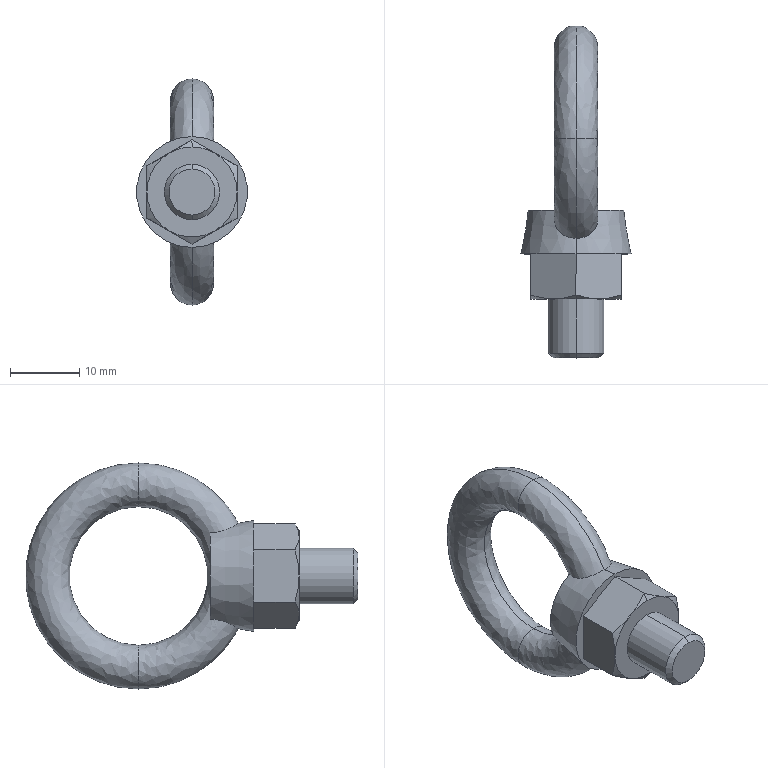Part | SolidWorks | features BaseBody 2 | 2 solids | 37 faces | box 16 x 47.95 x 32.6 mm | volume 4723 mm3 | cone 15 | plane 12 | spline 6 | cylinder 4 | commonest cylinder face diameters 6.647 x2 8 x2
STEP:
#1=CARTESIAN_POINT('',(0.,0.,-10.));
#2=VERTEX_POINT('',#1);
#3=CARTESIAN_POINT('',(0.,0.,10.));
#4=VERTEX_POINT('',#3);
#5=CARTESIAN_POINT('',(0.,0.,0.));
#6=DIRECTION('',(-1.,0.,0.));
#7=DIRECTION('',(0.,0.,1.));
#8=AXIS2_PLACEMENT_3D('',#5,#6,#7);
#9=CIRCLE('',#8,10.);
#10=EDGE_CURVE('',#2,#4,#9,.T.);
#11=ORIENTED_EDGE('',*,*,#10,.F.);
#12=CARTESIAN_POINT('',(0.,0.,-16.3));
#13=VERTEX_POINT('',#12);
#14=CARTESIAN_POINT('',(0.,0.,-13.15));
#15=DIRECTION('',(0.,-1.,0.));
#16=DIRECTION('',(0.,0.,-1.));
#17=AXIS2_PLACEMENT_3D('',#14,#15,#16);
#18=CIRCLE('',#17,3.15);
#19=EDGE_CURVE('',#2,#13,#18,.T.);
#20=ORIENTED_EDGE('',*,*,#19,.T.);
#21=CARTESIAN_POINT('',(0.,-14.417,-7.606));
#22=VERTEX_POINT('',#21);
#23=CARTESIAN_POINT('',(0.,0.,0.));
#24=DIRECTION('',(-1.,0.,0.));
#25=DIRECTION('',(0.,0.,1.));
#26=AXIS2_PLACEMENT_3D('',#23,#24,#25);
#27=CIRCLE('',#26,16.3);
#28=EDGE_CURVE('',#13,#22,#27,.T.);
#29=ORIENTED_EDGE('',*,*,#28,.T.);
#30=CARTESIAN_POINT('',(-2.961,-10.35,-6.22));
#31=VERTEX_POINT('',#30);
#32=CARTESIAN_POINT('',(0.,-14.417,-7.606));
#33=CARTESIAN_POINT('',(-0.2595,-14.417,-7.606));
#34=CARTESIAN_POINT('',(-0.5135,-14.39,-7.588));
#35=CARTESIAN_POINT('',(-1.011,-14.286,-7.52));
#36=CARTESIAN_POINT('',(-1.255,-14.207,-7.468));
#37=CARTESIAN_POINT('',(-1.594,-14.054,-7.373));
#38=CARTESIAN_POINT('',(-1.703,-13.996,-7.338));
#39=CARTESIAN_POINT('',(-1.913,-13.869,-7.263));
#40=CARTESIAN_POINT('',(-2.015,-13.799,-7.222));
#41=CARTESIAN_POINT('',(-2.302,-13.573,-7.096));
#42=CARTESIAN_POINT('',(-2.469,-13.402,-7.007));
#43=CARTESIAN_POINT('',(-2.757,-13.014,-6.825));
#44=CARTESIAN_POINT('',(-2.874,-12.801,-6.735));
#45=CARTESIAN_POINT('',(-3.047,-12.348,-6.57));
#46=CARTESIAN_POINT('',(-3.105,-12.104,-6.495));
#47=CARTESIAN_POINT('',(-3.158,-11.609,-6.372));
#48=CARTESIAN_POINT('',(-3.155,-11.354,-6.323));
#49=CARTESIAN_POINT('',(-3.096,-10.847,-6.252));
#50=CARTESIAN_POINT('',(-3.04,-10.597,-6.231));
#51=CARTESIAN_POINT('',(-2.961,-10.35,-6.22));
#52=B_SPLINE_CURVE_WITH_KNOTS('',3,(#32,#33,#34,#35,#36,#37,#38,#39,#40,#41,#42,#43,#44,#45,#46,#47,#48,#49,#50,#51),.UNSPECIFIED.,.F.,.F.,(4,2,2,2,2,2,2,2,2,4),(0.00614,0.006907,0.007674,0.008058,0.008441,0.009209,0.009976,0.01074,0.01151,0.01228),.UNSPECIFIED.);
#53=EDGE_CURVE('',#22,#31,#52,.T.);
#54=ORIENTED_EDGE('',*,*,#53,.T.);
#55=CARTESIAN_POINT('',(-2.961,-10.35,6.22));
#56=VERTEX_POINT('',#55);
#57=CARTESIAN_POINT('',(-2.961,-10.35,-6.22));
#58=CARTESIAN_POINT('',(-2.862,-10.35,-5.691));
#59=CARTESIAN_POINT('',(-2.732,-10.35,-5.171));
#60=CARTESIAN_POINT('',(-2.436,-10.35,-4.139));
#61=CARTESIAN_POINT('',(-2.271,-10.35,-3.628));
#62=CARTESIAN_POINT('',(-1.944,-10.35,-2.605));
#63=CARTESIAN_POINT('',(-1.78,-10.35,-2.093));
#64=CARTESIAN_POINT('',(-1.59,-10.35,-1.314));
#65=CARTESIAN_POINT('',(-1.537,-10.35,-1.052));
#66=CARTESIAN_POINT('',(-1.462,-10.35,-0.5207));
#67=CARTESIAN_POINT('',(-1.442,-10.35,-0.2495));
#68=CARTESIAN_POINT('',(-1.445,-10.35,0.5655));
#69=CARTESIAN_POINT('',(-1.534,-10.35,1.09));
#70=CARTESIAN_POINT('',(-1.789,-10.35,2.121));
#71=CARTESIAN_POINT('',(-1.952,-10.35,2.629));
#72=CARTESIAN_POINT('',(-2.277,-10.35,3.646));
#73=CARTESIAN_POINT('',(-2.441,-10.35,4.153));
#74=CARTESIAN_POINT('',(-2.733,-10.35,5.178));
#75=CARTESIAN_POINT('',(-2.863,-10.35,5.695));
#76=CARTESIAN_POINT('',(-2.961,-10.35,6.22));
#77=B_SPLINE_CURVE_WITH_KNOTS('',3,(#57,#58,#59,#60,#61,#62,#63,#64,#65,#66,#67,#68,#69,#70,#71,#72,#73,#74,#75,#76),.UNSPECIFIED.,.F.,.F.,(4,2,2,2,2,2,2,2,2,4),(0.,0.00161,0.003219,0.004829,0.005634,0.006439,0.008048,0.009658,0.01127,0.01288),.UNSPECIFIED.);
#78=EDGE_CURVE('',#31,#56,#77,.T.);
#79=ORIENTED_EDGE('',*,*,#78,.T.);
#80=CARTESIAN_POINT('',(0.,-14.417,7.606));
#81=VERTEX_POINT('',#80);
#82=CARTESIAN_POINT('',(-2.961,-10.35,6.22));
#83=CARTESIAN_POINT('',(-3.04,-10.596,6.231));
#84=CARTESIAN_POINT('',(-3.095,-10.846,6.252));
#85=CARTESIAN_POINT('',(-3.155,-11.35,6.322));
#86=CARTESIAN_POINT('',(-3.158,-11.607,6.371));
#87=CARTESIAN_POINT('',(-3.106,-12.1,6.493));
#88=CARTESIAN_POINT('',(-3.05,-12.34,6.567));
#89=CARTESIAN_POINT('',(-2.875,-12.798,6.734));
#90=CARTESIAN_POINT('',(-2.76,-13.009,6.823));
#91=CARTESIAN_POINT('',(-2.546,-13.299,6.959));
#92=CARTESIAN_POINT('',(-2.466,-13.392,7.005));
#93=CARTESIAN_POINT('',(-2.298,-13.566,7.094));
#94=CARTESIAN_POINT('',(-2.208,-13.646,7.137));
#95=CARTESIAN_POINT('',(-1.923,-13.872,7.263));
#96=CARTESIAN_POINT('',(-1.709,-14.001,7.34));
#97=CARTESIAN_POINT('',(-1.257,-14.206,7.468));
#98=CARTESIAN_POINT('',(-1.017,-14.285,7.519));
#99=CARTESIAN_POINT('',(-0.5148,-14.39,7.588));
#100=CARTESIAN_POINT('',(-0.2595,-14.417,7.606));
#101=CARTESIAN_POINT('',(0.,-14.417,7.606));
#102=B_SPLINE_CURVE_WITH_KNOTS('',3,(#82,#83,#84,#85,#86,#87,#88,#89,#90,#91,#92,#93,#94,#95,#96,#97,#98,#99,#100,#101),.UNSPECIFIED.,.F.,.F.,(4,2,2,2,2,2,2,2,2,4),(-0.00614,-0.005372,-0.004605,-0.003837,-0.00307,-0.002686,-0.002302,-0.001535,-0.0007674,0.),.UNSPECIFIED.);
#103=EDGE_CURVE('',#56,#81,#102,.T.);
#104=ORIENTED_EDGE('',*,*,#103,.T.);
#105=CARTESIAN_POINT('',(0.,0.,16.3));
#106=VERTEX_POINT('',#105);
#107=CARTESIAN_POINT('',(0.,0.,0.));
#108=DIRECTION('',(-1.,0.,0.));
#109=DIRECTION('',(0.,0.,1.));
#110=AXIS2_PLACEMENT_3D('',#107,#108,#109);
#111=CIRCLE('',#110,16.3);
#112=EDGE_CURVE('',#81,#106,#111,.T.);
#113=ORIENTED_EDGE('',*,*,#112,.T.);
#114=CARTESIAN_POINT('',(0.,0.,13.15));
#115=DIRECTION('',(0.,1.,0.));
#116=DIRECTION('',(0.,0.,1.));
#117=AXIS2_PLACEMENT_3D('',#114,#115,#116);
#118=CIRCLE('',#117,3.15);
#119=EDGE_CURVE('',#4,#106,#118,.T.);
#120=ORIENTED_EDGE('',*,*,#119,.F.);
#121=EDGE_LOOP('',(#11,#20,#29,#54,#79,#104,#113,#120));
#122=FACE_OUTER_BOUND('',#121,.T.);
#123=CARTESIAN_POINT('',(0.,0.,-10.));
#124=CARTESIAN_POINT('',(0.,-20.,-10.));
#125=CARTESIAN_POINT('',(0.,-20.,10.));
#126=CARTESIAN_POINT('',(0.,0.,10.));
#127=CARTESIAN_POINT('',(-6.3,0.,-10.));
#128=CARTESIAN_POINT('',(-6.3,-20.,-10.));
#129=CARTESIAN_POINT('',(-6.3,-20.,10.));
#130=CARTESIAN_POINT('',(-6.3,0.,10.));
#131=CARTESIAN_POINT('',(-6.3,0.,-16.3));
#132=CARTESIAN_POINT('',(-6.3,-32.6,-16.3));
#133=CARTESIAN_POINT('',(-6.3,-32.6,16.3));
#134=CARTESIAN_POINT('',(-6.3,0.,16.3));
#135=CARTESIAN_POINT('',(0.,0.,-16.3));
#136=CARTESIAN_POINT('',(0.,-32.6,-16.3));
#137=CARTESIAN_POINT('',(0.,-32.6,16.3));
#138=CARTESIAN_POINT('',(0.,0.,16.3));
#139=(BOUNDED_SURFACE()B_SPLINE_SURFACE(3,3,((#123,#124,#125,#126),(#127,#128,#129,#130),(#131,#132,#133,#134),(#135,#136,#137,#138)),.UNSPECIFIED.,.F.,.F.,.F.)B_SPLINE_SURFACE_WITH_KNOTS((4,4),(4,4),(0.,1.),(0.,1.),.UNSPECIFIED.)GEOMETRIC_REPRESENTATION_ITEM()RATIONAL_B_SPLINE_SURFACE(((1.,0.3333,0.3333,1.),(0.3333,0.1111,0.1111,0.3333),(0.3333,0.1111,0.1111,0.3333),(1.,0.3333,0.3333,1.)))REPRESENTATION_ITEM('')SURFACE());
#140=ADVANCED_FACE('',(#122),#139,.T.);
#141=CARTESIAN_POINT('',(0.,-19.65,-4.));
#142=VERTEX_POINT('',#141);
#143=CARTESIAN_POINT('',(0.,-19.65,4.));
#144=VERTEX_POINT('',#143);
#145=CARTESIAN_POINT('',(0.,-19.65,0.));
#146=DIRECTION('',(0.,-1.,0.));
#147=DIRECTION('',(0.,0.,1.));
#148=AXIS2_PLACEMENT_3D('',#145,#146,#147);
#149=CIRCLE('',#148,4.);
#150=EDGE_CURVE('',#142,#144,#149,.T.);
#151=ORIENTED_EDGE('',*,*,#150,.F.);
#152=CARTESIAN_POINT('',(0.,-16.65,-4.));
#153=VERTEX_POINT('',#152);
#154=CARTESIAN_POINT('',(0.,-18.15,-7.708));
#155=DIRECTION('',(-1.,0.,0.));
#156=DIRECTION('',(0.,0.,-1.));
#157=AXIS2_PLACEMENT_3D('',#154,#155,#156);
#158=CIRCLE('',#157,4.);
#159=EDGE_CURVE('',#142,#153,#158,.T.);
#160=ORIENTED_EDGE('',*,*,#159,.T.);
#161=CARTESIAN_POINT('',(0.,-16.65,4.));
#162=VERTEX_POINT('',#161);
#163=CARTESIAN_POINT('',(0.,-16.65,0.));
#164=DIRECTION('',(0.,1.,0.));
#165=DIRECTION('',(0.,0.,1.));
#166=AXIS2_PLACEMENT_3D('',#163,#164,#165);
#167=CIRCLE('',#166,4.);
#168=EDGE_CURVE('',#162,#153,#167,.T.);
#169=ORIENTED_EDGE('',*,*,#168,.F.);
#170=CARTESIAN_POINT('',(0.,-18.15,7.708));
#171=DIRECTION('',(1.,0.,0.));
#172=DIRECTION('',(0.,0.,1.));
#173=AXIS2_PLACEMENT_3D('',#170,#171,#172);
#174=CIRCLE('',#173,4.);
#175=EDGE_CURVE('',#144,#162,#174,.T.);
#176=ORIENTED_EDGE('',*,*,#175,.F.);
#177=EDGE_LOOP('',(#151,#160,#169,#176));
#178=FACE_OUTER_BOUND('',#177,.T.);
#179=CARTESIAN_POINT('',(0.,-19.65,4.));
#180=CARTESIAN_POINT('',(8.,-19.65,4.));
#181=CARTESIAN_POINT('',(8.,-19.65,-4.));
#182=CARTESIAN_POINT('',(0.,-19.65,-4.));
#183=CARTESIAN_POINT('',(0.,-18.676,3.606));
#184=CARTESIAN_POINT('',(7.212,-18.676,3.606));
#185=CARTESIAN_POINT('',(7.212,-18.676,-3.606));
#186=CARTESIAN_POINT('',(0.,-18.676,-3.606));
#187=CARTESIAN_POINT('',(0.,-17.624,3.606));
#188=CARTESIAN_POINT('',(7.212,-17.624,3.606));
#189=CARTESIAN_POINT('',(7.212,-17.624,-3.606));
#190=CARTESIAN_POINT('',(0.,-17.624,-3.606));
#191=CARTESIAN_POINT('',(0.,-16.65,4.));
#192=CARTESIAN_POINT('',(8.,-16.65,4.));
#193=CARTESIAN_POINT('',(8.,-16.65,-4.));
#194=CARTESIAN_POINT('',(0.,-16.65,-4.));
#195=(BOUNDED_SURFACE()B_SPLINE_SURFACE(3,3,((#179,#180,#181,#182),(#183,#184,#185,#186),(#187,#188,#189,#190),(#191,#192,#193,#194)),.UNSPECIFIED.,.F.,.F.,.F.)B_SPLINE_SURFACE_WITH_KNOTS((4,4),(4,4),(0.,1.),(0.,1.),.UNSPECIFIED.)GEOMETRIC_REPRESENTATION_ITEM()RATIONAL_B_SPLINE_SURFACE(((1.,0.3333,0.3333,1.),(0.9513,0.3171,0.3171,0.9513),(0.9513,0.3171,0.3171,0.9513),(1.,0.3333,0.3333,1.)))REPRESENTATION_ITEM('')SURFACE());
#196=ADVANCED_FACE('',(#178),#195,.F.);
#197=ORIENTED_EDGE('',*,*,#28,.F.);
#198=CARTESIAN_POINT('',(0.,0.,-13.15));
#199=DIRECTION('',(0.,-1.,0.));
#200=DIRECTION('',(0.,0.,-1.));
#201=AXIS2_PLACEMENT_3D('',#198,#199,#200);
#202=CIRCLE('',#201,3.15);
#203=EDGE_CURVE('',#13,#2,#202,.T.);
#204=ORIENTED_EDGE('',*,*,#203,.T.);
#205=ORIENTED_EDGE('',*,*,#10,.T.);
#206=CARTESIAN_POINT('',(0.,0.,13.15));
#207=DIRECTION('',(0.,1.,0.));
#208=DIRECTION('',(0.,0.,1.));
#209=AXIS2_PLACEMENT_3D('',#206,#207,#208);
#210=CIRCLE('',#209,3.15);
#211=EDGE_CURVE('',#106,#4,#210,.T.);
#212=ORIENTED_EDGE('',*,*,#211,.F.);
#213=ORIENTED_EDGE('',*,*,#112,.F.);
#214=CARTESIAN_POINT('',(2.961,-10.35,6.22));
#215=VERTEX_POINT('',#214);
#216=CARTESIAN_POINT('',(0.,-14.417,7.606));
#217=CARTESIAN_POINT('',(0.2595,-14.417,7.606));
#218=CARTESIAN_POINT('',(0.5135,-14.39,7.588));
#219=CARTESIAN_POINT('',(1.011,-14.286,7.52));
#220=CARTESIAN_POINT('',(1.255,-14.207,7.468));
#221=CARTESIAN_POINT('',(1.594,-14.054,7.373));
#222=CARTESIAN_POINT('',(1.703,-13.996,7.338));
#223=CARTESIAN_POINT('',(1.913,-13.869,7.263));
#224=CARTESIAN_POINT('',(2.015,-13.799,7.222));
#225=CARTESIAN_POINT('',(2.302,-13.573,7.096));
#226=CARTESIAN_POINT('',(2.469,-13.402,7.007));
#227=CARTESIAN_POINT('',(2.757,-13.014,6.825));
#228=CARTESIAN_POINT('',(2.874,-12.801,6.735));
#229=CARTESIAN_POINT('',(3.047,-12.348,6.57));
#230=CARTESIAN_POINT('',(3.105,-12.104,6.495));
#231=CARTESIAN_POINT('',(3.158,-11.609,6.372));
#232=CARTESIAN_POINT('',(3.155,-11.354,6.323));
#233=CARTESIAN_POINT('',(3.096,-10.847,6.252));
#234=CARTESIAN_POINT('',(3.04,-10.597,6.231));
#235=CARTESIAN_POINT('',(2.961,-10.35,6.22));
#236=B_SPLINE_CURVE_WITH_KNOTS('',3,(#216,#217,#218,#219,#220,#221,#222,#223,#224,#225,#226,#227,#228,#229,#230,#231,#232,#233,#234,#235),.UNSPECIFIED.,.F.,.F.,(4,2,2,2,2,2,2,2,2,4),(0.,0.0007672,0.001534,0.001918,0.002302,0.003069,0.003836,0.004603,0.005371,0.006138),.UNSPECIFIED.);
#237=EDGE_CURVE('',#81,#215,#236,.T.);
#238=ORIENTED_EDGE('',*,*,#237,.T.);
#239=CARTESIAN_POINT('',(2.961,-10.35,-6.22));
#240=VERTEX_POINT('',#239);
#241=CARTESIAN_POINT('',(2.961,-10.35,6.22));
#242=CARTESIAN_POINT('',(2.862,-10.35,5.691));
#243=CARTESIAN_POINT('',(2.732,-10.35,5.171));
#244=CARTESIAN_POINT('',(2.436,-10.35,4.139));
#245=CARTESIAN_POINT('',(2.271,-10.35,3.628));
#246=CARTESIAN_POINT('',(1.944,-10.35,2.605));
#247=CARTESIAN_POINT('',(1.78,-10.35,2.093));
#248=CARTESIAN_POINT('',(1.59,-10.35,1.314));
#249=CARTESIAN_POINT('',(1.537,-10.35,1.052));
#250=CARTESIAN_POINT('',(1.462,-10.35,0.5207));
#251=CARTESIAN_POINT('',(1.442,-10.35,0.2495));
#252=CARTESIAN_POINT('',(1.445,-10.35,-0.5655));
#253=CARTESIAN_POINT('',(1.534,-10.35,-1.09));
#254=CARTESIAN_POINT('',(1.789,-10.35,-2.121));
#255=CARTESIAN_POINT('',(1.952,-10.35,-2.629));
#256=CARTESIAN_POINT('',(2.277,-10.35,-3.646));
#257=CARTESIAN_POINT('',(2.441,-10.35,-4.153));
#258=CARTESIAN_POINT('',(2.733,-10.35,-5.178));
#259=CARTESIAN_POINT('',(2.863,-10.35,-5.695));
#260=CARTESIAN_POINT('',(2.961,-10.35,-6.22));
#261=B_SPLINE_CURVE_WITH_KNOTS('',3,(#241,#242,#243,#244,#245,#246,#247,#248,#249,#250,#251,#252,#253,#254,#255,#256,#257,#258,#259,#260),.UNSPECIFIED.,.F.,.F.,(4,2,2,2,2,2,2,2,2,4),(0.,0.00161,0.003219,0.004829,0.005634,0.006439,0.008048,0.009658,0.01127,0.01288),.UNSPECIFIED.);
#262=EDGE_CURVE('',#215,#240,#261,.T.);
#263=ORIENTED_EDGE('',*,*,#262,.T.);
#264=CARTESIAN_POINT('',(2.961,-10.35,-6.22));
#265=CARTESIAN_POINT('',(3.04,-10.596,-6.231));
#266=CARTESIAN_POINT('',(3.095,-10.846,-6.252));
#267=CARTESIAN_POINT('',(3.155,-11.35,-6.322));
#268=CARTESIAN_POINT('',(3.158,-11.607,-6.371));
#269=CARTESIAN_POINT('',(3.106,-12.1,-6.493));
#270=CARTESIAN_POINT('',(3.05,-12.34,-6.567));
#271=CARTESIAN_POINT('',(2.875,-12.798,-6.734));
#272=CARTESIAN_POINT('',(2.76,-13.009,-6.823));
#273=CARTESIAN_POINT('',(2.546,-13.299,-6.959));
#274=CARTESIAN_POINT('',(2.466,-13.392,-7.005));
#275=CARTESIAN_POINT('',(2.298,-13.566,-7.094));
#276=CARTESIAN_POINT('',(2.208,-13.646,-7.137));
#277=CARTESIAN_POINT('',(1.923,-13.872,-7.263));
#278=CARTESIAN_POINT('',(1.709,-14.001,-7.34));
#279=CARTESIAN_POINT('',(1.257,-14.206,-7.468));
#280=CARTESIAN_POINT('',(1.017,-14.285,-7.519));
#281=CARTESIAN_POINT('',(0.5148,-14.39,-7.588));
#282=CARTESIAN_POINT('',(0.2595,-14.417,-7.606));
#283=CARTESIAN_POINT('',(0.,-14.417,-7.606));
#284=B_SPLINE_CURVE_WITH_KNOTS('',3,(#264,#265,#266,#267,#268,#269,#270,#271,#272,#273,#274,#275,#276,#277,#278,#279,#280,#281,#282,#283),.UNSPECIFIED.,.F.,.F.,(4,2,2,2,2,2,2,2,2,4),(0.,0.0007675,0.001535,0.002302,0.00307,0.003454,0.003837,0.004605,0.005372,0.00614),.UNSPECIFIED.);
#285=EDGE_CURVE('',#240,#22,#284,.T.);
#286=ORIENTED_EDGE('',*,*,#285,.T.);
#287=EDGE_LOOP('',(#197,#204,#205,#212,#213,#238,#263,#286));
#288=FACE_OUTER_BOUND('',#287,.T.);
#289=CARTESIAN_POINT('',(0.,0.,-16.3));
#290=CARTESIAN_POINT('',(0.,-32.6,-16.3));
#291=CARTESIAN_POINT('',(0.,-32.6,16.3));
#292=CARTESIAN_POINT('',(0.,0.,16.3));
#293=CARTESIAN_POINT('',(6.3,0.,-16.3));
#294=CARTESIAN_POINT('',(6.3,-32.6,-16.3));
#295=CARTESIAN_POINT('',(6.3,-32.6,16.3));
#296=CARTESIAN_POINT('',(6.3,0.,16.3));
#297=CARTESIAN_POINT('',(6.3,0.,-10.));
#298=CARTESIAN_POINT('',(6.3,-20.,-10.));
#299=CARTESIAN_POINT('',(6.3,-20.,10.));
#300=CARTESIAN_POINT('',(6.3,0.,10.));
#301=CARTESIAN_POINT('',(0.,0.,-10.));
#302=CARTESIAN_POINT('',(0.,-20.,-10.));
#303=CARTESIAN_POINT('',(0.,-20.,10.));
#304=CARTESIAN_POINT('',(0.,0.,10.));
#305=(BOUNDED_SURFACE()B_SPLINE_SURFACE(3,3,((#289,#290,#291,#292),(#293,#294,#295,#296),(#297,#298,#299,#300),(#301,#302,#303,#304)),.UNSPECIFIED.,.F.,.F.,.F.)B_SPLINE_SURFACE_WITH_KNOTS((4,4),(4,4),(0.,1.),(0.,1.),.UNSPECIFIED.)GEOMETRIC_REPRESENTATION_ITEM()RATIONAL_B_SPLINE_SURFACE(((1.,0.3333,0.3333,1.),(0.3333,0.1111,0.1111,0.3333),(0.3333,0.1111,0.1111,0.3333),(1.,0.3333,0.3333,1.)))REPRESENTATION_ITEM('')SURFACE());
#306=ADVANCED_FACE('',(#288),#305,.T.);
#307=ORIENTED_EDGE('',*,*,#203,.F.);
#308=CARTESIAN_POINT('',(0.,0.,0.));
#309=DIRECTION('',(-1.,0.,0.));
#310=DIRECTION('',(0.,0.,1.));
#311=AXIS2_PLACEMENT_3D('',#308,#309,#310);
#312=CIRCLE('',#311,16.3);
#313=EDGE_CURVE('',#106,#13,#312,.T.);
#314=ORIENTED_EDGE('',*,*,#313,.F.);
#315=ORIENTED_EDGE('',*,*,#211,.T.);
#316=CARTESIAN_POINT('',(0.,0.,0.));
#317=DIRECTION('',(-1.,0.,0.));
#318=DIRECTION('',(0.,0.,1.));
#319=AXIS2_PLACEMENT_3D('',#316,#317,#318);
#320=CIRCLE('',#319,10.);
#321=EDGE_CURVE('',#4,#2,#320,.T.);
#322=ORIENTED_EDGE('',*,*,#321,.T.);
#323=EDGE_LOOP('',(#307,#314,#315,#322));
#324=FACE_OUTER_BOUND('',#323,.T.);
#325=CARTESIAN_POINT('',(0.,0.,16.3));
#326=CARTESIAN_POINT('',(0.,32.6,16.3));
#327=CARTESIAN_POINT('',(0.,32.6,-16.3));
#328=CARTESIAN_POINT('',(0.,0.,-16.3));
#329=CARTESIAN_POINT('',(6.3,0.,16.3));
#330=CARTESIAN_POINT('',(6.3,32.6,16.3));
#331=CARTESIAN_POINT('',(6.3,32.6,-16.3));
#332=CARTESIAN_POINT('',(6.3,0.,-16.3));
#333=CARTESIAN_POINT('',(6.3,0.,10.));
#334=CARTESIAN_POINT('',(6.3,20.,10.));
#335=CARTESIAN_POINT('',(6.3,20.,-10.));
#336=CARTESIAN_POINT('',(6.3,0.,-10.));
#337=CARTESIAN_POINT('',(0.,0.,10.));
#338=CARTESIAN_POINT('',(0.,20.,10.));
#339=CARTESIAN_POINT('',(0.,20.,-10.));
#340=CARTESIAN_POINT('',(0.,0.,-10.));
#341=(BOUNDED_SURFACE()B_SPLINE_SURFACE(3,3,((#325,#326,#327,#328),(#329,#330,#331,#332),(#333,#334,#335,#336),(#337,#338,#339,#340)),.UNSPECIFIED.,.F.,.F.,.F.)B_SPLINE_SURFACE_WITH_KNOTS((4,4),(4,4),(0.,1.),(0.,1.),.UNSPECIFIED.)GEOMETRIC_REPRESENTATION_ITEM()RATIONAL_B_SPLINE_SURFACE(((1.,0.3333,0.3333,1.),(0.3333,0.1111,0.1111,0.3333),(0.3333,0.1111,0.1111,0.3333),(1.,0.3333,0.3333,1.)))REPRESENTATION_ITEM('')SURFACE());
#342=ADVANCED_FACE('',(#324),#341,.T.);
#343=ORIENTED_EDGE('',*,*,#237,.F.);
#344=CARTESIAN_POINT('',(0.,-16.65,8.));
#345=VERTEX_POINT('',#344);
#346=CARTESIAN_POINT('',(0.,-16.65,8.));
#347=DIRECTION('',(0.,-0.9848,0.1736));
#348=VECTOR('',#347,1000.);
#349=LINE('',#346,#348);
#350=EDGE_CURVE('',#81,#345,#349,.T.);
#351=ORIENTED_EDGE('',*,*,#350,.T.);
#352=CARTESIAN_POINT('',(0.,-16.65,-8.));
#353=VERTEX_POINT('',#352);
#354=CARTESIAN_POINT('',(0.,-16.65,0.));
#355=DIRECTION('',(0.,1.,0.));
#356=DIRECTION('',(0.,0.,-1.));
#357=AXIS2_PLACEMENT_3D('',#354,#355,#356);
#358=CIRCLE('',#357,8.);
#359=EDGE_CURVE('',#345,#353,#358,.T.);
#360=ORIENTED_EDGE('',*,*,#359,.T.);
#361=CARTESIAN_POINT('',(0.,-16.65,-8.));
#362=DIRECTION('',(0.,-0.9848,-0.1736));
#363=VECTOR('',#362,1000.);
#364=LINE('',#361,#363);
#365=EDGE_CURVE('',#22,#353,#364,.T.);
#366=ORIENTED_EDGE('',*,*,#365,.F.);
#367=ORIENTED_EDGE('',*,*,#285,.F.);
#368=CARTESIAN_POINT('',(0.,-10.35,0.));
#369=DIRECTION('',(0.,-1.,0.));
#370=DIRECTION('',(0.,0.,-1.));
#371=AXIS2_PLACEMENT_3D('',#368,#369,#370);
#372=CIRCLE('',#371,6.889);
#373=EDGE_CURVE('',#240,#215,#372,.T.);
#374=ORIENTED_EDGE('',*,*,#373,.T.);
#375=EDGE_LOOP('',(#343,#351,#360,#366,#367,#374));
#376=FACE_OUTER_BOUND('',#375,.T.);
#377=CARTESIAN_POINT('',(0.,-16.65,0.));
#378=DIRECTION('',(0.,-1.,0.));
#379=DIRECTION('',(0.,0.,-1.));
#380=AXIS2_PLACEMENT_3D('',#377,#378,#379);
#381=CONICAL_SURFACE('',#380,8.,0.1745);
#382=ADVANCED_FACE('',(#376),#381,.T.);
#383=ORIENTED_EDGE('',*,*,#150,.T.);
#384=CARTESIAN_POINT('',(0.,-30.974,4.));
#385=VERTEX_POINT('',#384);
#386=CARTESIAN_POINT('',(0.,-25.312,4.));
#387=DIRECTION('',(0.,-1.,0.));
#388=VECTOR('',#387,1000.);
#389=LINE('',#386,#388);
#390=EDGE_CURVE('',#144,#385,#389,.T.);
#391=ORIENTED_EDGE('',*,*,#390,.T.);
#392=CARTESIAN_POINT('',(0.,-30.974,-4.));
#393=VERTEX_POINT('',#392);
#394=CARTESIAN_POINT('',(0.,-30.974,0.));
#395=DIRECTION('',(0.,1.,0.));
#396=DIRECTION('',(0.,0.,-1.));
#397=AXIS2_PLACEMENT_3D('',#394,#395,#396);
#398=CIRCLE('',#397,4.);
#399=EDGE_CURVE('',#385,#393,#398,.T.);
#400=ORIENTED_EDGE('',*,*,#399,.T.);
#401=CARTESIAN_POINT('',(0.,-25.312,-4.));
#402=DIRECTION('',(0.,-1.,0.));
#403=VECTOR('',#402,1000.);
#404=LINE('',#401,#403);
#405=EDGE_CURVE('',#142,#393,#404,.T.);
#406=ORIENTED_EDGE('',*,*,#405,.F.);
#407=EDGE_LOOP('',(#383,#391,#400,#406));
#408=FACE_OUTER_BOUND('',#407,.T.);
#409=CARTESIAN_POINT('',(0.,-25.312,0.));
#410=DIRECTION('',(0.,-1.,0.));
#411=DIRECTION('',(0.,0.,-1.));
#412=AXIS2_PLACEMENT_3D('',#409,#410,#411);
#413=CYLINDRICAL_SURFACE('',#412,4.);
#414=ADVANCED_FACE('',(#408),#413,.T.);
#415=CARTESIAN_POINT('',(0.,-31.65,3.324));
#416=VERTEX_POINT('',#415);
#417=CARTESIAN_POINT('',(0.,-31.65,-3.324));
#418=VERTEX_POINT('',#417);
#419=CARTESIAN_POINT('',(0.,-31.65,0.));
#420=DIRECTION('',(0.,1.,0.));
#421=DIRECTION('',(0.,0.,1.));
#422=AXIS2_PLACEMENT_3D('',#419,#420,#421);
#423=CIRCLE('',#422,3.324);
#424=EDGE_CURVE('',#416,#418,#423,.T.);
#425=ORIENTED_EDGE('',*,*,#424,.T.);
#426=CARTESIAN_POINT('',(0.,-30.974,-4.));
#427=DIRECTION('',(0.,0.7071,-0.7071));
#428=VECTOR('',#427,1000.);
#429=LINE('',#426,#428);
#430=EDGE_CURVE('',#418,#393,#429,.T.);
#431=ORIENTED_EDGE('',*,*,#430,.T.);
#432=ORIENTED_EDGE('',*,*,#399,.F.);
#433=CARTESIAN_POINT('',(0.,-30.974,4.));
#434=DIRECTION('',(0.,0.7071,0.7071));
#435=VECTOR('',#434,1000.);
#436=LINE('',#433,#435);
#437=EDGE_CURVE('',#416,#385,#436,.T.);
#438=ORIENTED_EDGE('',*,*,#437,.F.);
#439=EDGE_LOOP('',(#425,#431,#432,#438));
#440=FACE_OUTER_BOUND('',#439,.T.);
#441=CARTESIAN_POINT('',(0.,-30.974,0.));
#442=DIRECTION('',(0.,1.,0.));
#443=DIRECTION('',(0.,0.,1.));
#444=AXIS2_PLACEMENT_3D('',#441,#442,#443);
#445=CONICAL_SURFACE('',#444,4.,0.7854);
#446=ADVANCED_FACE('',(#440),#445,.T.);
#447=ORIENTED_EDGE('',*,*,#19,.F.);
#448=ORIENTED_EDGE('',*,*,#321,.F.);
#449=ORIENTED_EDGE('',*,*,#119,.T.);
#450=ORIENTED_EDGE('',*,*,#313,.T.);
#451=EDGE_LOOP('',(#447,#448,#449,#450));
#452=FACE_OUTER_BOUND('',#451,.T.);
#453=CARTESIAN_POINT('',(0.,0.,10.));
#454=CARTESIAN_POINT('',(0.,20.,10.));
#455=CARTESIAN_POINT('',(0.,20.,-10.));
#456=CARTESIAN_POINT('',(0.,0.,-10.));
#457=CARTESIAN_POINT('',(-6.3,0.,10.));
#458=CARTESIAN_POINT('',(-6.3,20.,10.));
#459=CARTESIAN_POINT('',(-6.3,20.,-10.));
#460=CARTESIAN_POINT('',(-6.3,0.,-10.));
#461=CARTESIAN_POINT('',(-6.3,0.,16.3));
#462=CARTESIAN_POINT('',(-6.3,32.6,16.3));
#463=CARTESIAN_POINT('',(-6.3,32.6,-16.3));
#464=CARTESIAN_POINT('',(-6.3,0.,-16.3));
#465=CARTESIAN_POINT('',(0.,0.,16.3));
#466=CARTESIAN_POINT('',(0.,32.6,16.3));
#467=CARTESIAN_POINT('',(0.,32.6,-16.3));
#468=CARTESIAN_POINT('',(0.,0.,-16.3));
#469=(BOUNDED_SURFACE()B_SPLINE_SURFACE(3,3,((#453,#454,#455,#456),(#457,#458,#459,#460),(#461,#462,#463,#464),(#465,#466,#467,#468)),.UNSPECIFIED.,.F.,.F.,.F.)B_SPLINE_SURFACE_WITH_KNOTS((4,4),(4,4),(0.,1.),(0.,1.),.UNSPECIFIED.)GEOMETRIC_REPRESENTATION_ITEM()RATIONAL_B_SPLINE_SURFACE(((1.,0.3333,0.3333,1.),(0.3333,0.1111,0.1111,0.3333),(0.3333,0.1111,0.1111,0.3333),(1.,0.3333,0.3333,1.)))REPRESENTATION_ITEM('')SURFACE());
#470=ADVANCED_FACE('',(#452),#469,.T.);
#471=ORIENTED_EDGE('',*,*,#350,.F.);
#472=ORIENTED_EDGE('',*,*,#103,.F.);
#473=CARTESIAN_POINT('',(0.,-10.35,0.));
#474=DIRECTION('',(0.,-1.,0.));
#475=DIRECTION('',(0.,0.,-1.));
#476=AXIS2_PLACEMENT_3D('',#473,#474,#475);
#477=CIRCLE('',#476,6.889);
#478=EDGE_CURVE('',#56,#31,#477,.T.);
#479=ORIENTED_EDGE('',*,*,#478,.T.);
#480=ORIENTED_EDGE('',*,*,#53,.F.);
#481=ORIENTED_EDGE('',*,*,#365,.T.);
#482=CARTESIAN_POINT('',(0.,-16.65,0.));
#483=DIRECTION('',(0.,1.,0.));
#484=DIRECTION('',(0.,0.,-1.));
#485=AXIS2_PLACEMENT_3D('',#482,#483,#484);
#486=CIRCLE('',#485,8.);
#487=EDGE_CURVE('',#353,#345,#486,.T.);
#488=ORIENTED_EDGE('',*,*,#487,.T.);
#489=EDGE_LOOP('',(#471,#472,#479,#480,#481,#488));
#490=FACE_OUTER_BOUND('',#489,.T.);
#491=CARTESIAN_POINT('',(0.,-16.65,0.));
#492=DIRECTION('',(0.,-1.,0.));
#493=DIRECTION('',(0.,0.,-1.));
#494=AXIS2_PLACEMENT_3D('',#491,#492,#493);
#495=CONICAL_SURFACE('',#494,8.,0.1745);
#496=ADVANCED_FACE('',(#490),#495,.T.);
#497=ORIENTED_EDGE('',*,*,#262,.F.);
#498=ORIENTED_EDGE('',*,*,#373,.F.);
#499=EDGE_LOOP('',(#497,#498));
#500=FACE_OUTER_BOUND('',#499,.T.);
#501=CARTESIAN_POINT('',(0.,-10.35,-3.445));
#502=DIRECTION('',(0.,1.,0.));
#503=DIRECTION('',(0.,0.,1.));
#504=AXIS2_PLACEMENT_3D('',#501,#502,#503);
#505=PLANE('',#504);
#506=ADVANCED_FACE('',(#500),#505,.T.);
#507=ORIENTED_EDGE('',*,*,#78,.F.);
#508=ORIENTED_EDGE('',*,*,#478,.F.);
#509=EDGE_LOOP('',(#507,#508));
#510=FACE_OUTER_BOUND('',#509,.T.);
#511=CARTESIAN_POINT('',(0.,-10.35,-3.445));
#512=DIRECTION('',(0.,1.,0.));
#513=DIRECTION('',(0.,0.,1.));
#514=AXIS2_PLACEMENT_3D('',#511,#512,#513);
#515=PLANE('',#514);
#516=ADVANCED_FACE('',(#510),#515,.T.);
#517=ORIENTED_EDGE('',*,*,#168,.T.);
#518=CARTESIAN_POINT('',(0.,-16.65,0.));
#519=DIRECTION('',(0.,1.,0.));
#520=DIRECTION('',(0.,0.,1.));
#521=AXIS2_PLACEMENT_3D('',#518,#519,#520);
#522=CIRCLE('',#521,4.);
#523=EDGE_CURVE('',#153,#162,#522,.T.);
#524=ORIENTED_EDGE('',*,*,#523,.T.);
#525=EDGE_LOOP('',(#517,#524));
#526=FACE_BOUND('',#525,.T.);
#527=ORIENTED_EDGE('',*,*,#487,.F.);
#528=ORIENTED_EDGE('',*,*,#359,.F.);
#529=EDGE_LOOP('',(#527,#528));
#530=FACE_OUTER_BOUND('',#529,.T.);
#531=CARTESIAN_POINT('',(0.,-16.65,-6.));
#532=DIRECTION('',(0.,-1.,0.));
#533=DIRECTION('',(0.,0.,-1.));
#534=AXIS2_PLACEMENT_3D('',#531,#532,#533);
#535=PLANE('',#534);
#536=ADVANCED_FACE('',(#526,#530),#535,.T.);
#537=ORIENTED_EDGE('',*,*,#159,.F.);
#538=CARTESIAN_POINT('',(0.,-19.65,0.));
#539=DIRECTION('',(0.,-1.,0.));
#540=DIRECTION('',(0.,0.,1.));
#541=AXIS2_PLACEMENT_3D('',#538,#539,#540);
#542=CIRCLE('',#541,4.);
#543=EDGE_CURVE('',#144,#142,#542,.T.);
#544=ORIENTED_EDGE('',*,*,#543,.F.);
#545=ORIENTED_EDGE('',*,*,#175,.T.);
#546=ORIENTED_EDGE('',*,*,#523,.F.);
#547=EDGE_LOOP('',(#537,#544,#545,#546));
#548=FACE_OUTER_BOUND('',#547,.T.);
#549=CARTESIAN_POINT('',(0.,-19.65,-4.));
#550=CARTESIAN_POINT('',(-8.,-19.65,-4.));
#551=CARTESIAN_POINT('',(-8.,-19.65,4.));
#552=CARTESIAN_POINT('',(0.,-19.65,4.));
#553=CARTESIAN_POINT('',(0.,-18.676,-3.606));
#554=CARTESIAN_POINT('',(-7.212,-18.676,-3.606));
#555=CARTESIAN_POINT('',(-7.212,-18.676,3.606));
#556=CARTESIAN_POINT('',(0.,-18.676,3.606));
#557=CARTESIAN_POINT('',(0.,-17.624,-3.606));
#558=CARTESIAN_POINT('',(-7.212,-17.624,-3.606));
#559=CARTESIAN_POINT('',(-7.212,-17.624,3.606));
#560=CARTESIAN_POINT('',(0.,-17.624,3.606));
#561=CARTESIAN_POINT('',(0.,-16.65,-4.));
#562=CARTESIAN_POINT('',(-8.,-16.65,-4.));
#563=CARTESIAN_POINT('',(-8.,-16.65,4.));
#564=CARTESIAN_POINT('',(0.,-16.65,4.));
#565=(BOUNDED_SURFACE()B_SPLINE_SURFACE(3,3,((#549,#550,#551,#552),(#553,#554,#555,#556),(#557,#558,#559,#560),(#561,#562,#563,#564)),.UNSPECIFIED.,.F.,.F.,.F.)B_SPLINE_SURFACE_WITH_KNOTS((4,4),(4,4),(0.,1.),(0.,1.),.UNSPECIFIED.)GEOMETRIC_REPRESENTATION_ITEM()RATIONAL_B_SPLINE_SURFACE(((1.,0.3333,0.3333,1.),(0.9513,0.3171,0.3171,0.9513),(0.9513,0.3171,0.3171,0.9513),(1.,0.3333,0.3333,1.)))REPRESENTATION_ITEM('')SURFACE());
#566=ADVANCED_FACE('',(#548),#565,.F.);
#567=ORIENTED_EDGE('',*,*,#390,.F.);
#568=ORIENTED_EDGE('',*,*,#543,.T.);
#569=ORIENTED_EDGE('',*,*,#405,.T.);
#570=CARTESIAN_POINT('',(0.,-30.974,0.));
#571=DIRECTION('',(0.,1.,0.));
#572=DIRECTION('',(0.,0.,-1.));
#573=AXIS2_PLACEMENT_3D('',#570,#571,#572);
#574=CIRCLE('',#573,4.);
#575=EDGE_CURVE('',#393,#385,#574,.T.);
#576=ORIENTED_EDGE('',*,*,#575,.T.);
#577=EDGE_LOOP('',(#567,#568,#569,#576));
#578=FACE_OUTER_BOUND('',#577,.T.);
#579=CARTESIAN_POINT('',(0.,-25.312,0.));
#580=DIRECTION('',(0.,-1.,0.));
#581=DIRECTION('',(0.,0.,-1.));
#582=AXIS2_PLACEMENT_3D('',#579,#580,#581);
#583=CYLINDRICAL_SURFACE('',#582,4.);
#584=ADVANCED_FACE('',(#578),#583,.T.);
#585=ORIENTED_EDGE('',*,*,#430,.F.);
#586=CARTESIAN_POINT('',(0.,-31.65,0.));
#587=DIRECTION('',(0.,1.,0.));
#588=DIRECTION('',(0.,0.,1.));
#589=AXIS2_PLACEMENT_3D('',#586,#587,#588);
#590=CIRCLE('',#589,3.324);
#591=EDGE_CURVE('',#418,#416,#590,.T.);
#592=ORIENTED_EDGE('',*,*,#591,.T.);
#593=ORIENTED_EDGE('',*,*,#437,.T.);
#594=ORIENTED_EDGE('',*,*,#575,.F.);
#595=EDGE_LOOP('',(#585,#592,#593,#594));
#596=FACE_OUTER_BOUND('',#595,.T.);
#597=CARTESIAN_POINT('',(0.,-30.974,0.));
#598=DIRECTION('',(0.,1.,0.));
#599=DIRECTION('',(0.,0.,1.));
#600=AXIS2_PLACEMENT_3D('',#597,#598,#599);
#601=CONICAL_SURFACE('',#600,4.,0.7854);
#602=ADVANCED_FACE('',(#596),#601,.T.);
#603=ORIENTED_EDGE('',*,*,#424,.F.);
#604=ORIENTED_EDGE('',*,*,#591,.F.);
#605=EDGE_LOOP('',(#603,#604));
#606=FACE_OUTER_BOUND('',#605,.T.);
#607=CARTESIAN_POINT('',(0.,-31.65,-1.662));
#608=DIRECTION('',(0.,-1.,0.));
#609=DIRECTION('',(0.,0.,-1.));
#610=AXIS2_PLACEMENT_3D('',#607,#608,#609);
#611=PLANE('',#610);
#612=ADVANCED_FACE('',(#606),#611,.T.);
#613=CLOSED_SHELL('',(#140,#196,#306,#342,#382,#414,#446,#470,#496,#506,#516,#536,#566,#584,#602,#612));
#614=MANIFOLD_SOLID_BREP('',#613);
#615=CARTESIAN_POINT('',(0.,-17.326,-3.324));
#616=VERTEX_POINT('',#615);
#617=CARTESIAN_POINT('',(0.,-17.326,3.324));
#618=VERTEX_POINT('',#617);
#619=CARTESIAN_POINT('',(0.,-17.326,0.));
#620=DIRECTION('',(0.,1.,0.));
#621=DIRECTION('',(1.,0.,0.));
#622=AXIS2_PLACEMENT_3D('',#619,#620,#621);
#623=CIRCLE('',#622,3.324);
#624=EDGE_CURVE('',#616,#618,#623,.T.);
#625=ORIENTED_EDGE('',*,*,#624,.F.);
#626=CARTESIAN_POINT('',(0.,-16.65,-4.));
#627=VERTEX_POINT('',#626);
#628=CARTESIAN_POINT('',(0.,-16.65,-4.));
#629=DIRECTION('',(0.,0.7071,-0.7071));
#630=VECTOR('',#629,1000.);
#631=LINE('',#628,#630);
#632=EDGE_CURVE('',#616,#627,#631,.T.);
#633=ORIENTED_EDGE('',*,*,#632,.T.);
#634=CARTESIAN_POINT('',(0.,-16.65,4.));
#635=VERTEX_POINT('',#634);
#636=CARTESIAN_POINT('',(0.,-16.65,0.));
#637=DIRECTION('',(0.,-1.,0.));
#638=DIRECTION('',(0.,0.,1.));
#639=AXIS2_PLACEMENT_3D('',#636,#637,#638);
#640=CIRCLE('',#639,4.);
#641=EDGE_CURVE('',#635,#627,#640,.T.);
#642=ORIENTED_EDGE('',*,*,#641,.F.);
#643=CARTESIAN_POINT('',(0.,-16.65,4.));
#644=DIRECTION('',(0.,0.7071,0.7071));
#645=VECTOR('',#644,1000.);
#646=LINE('',#643,#645);
#647=EDGE_CURVE('',#618,#635,#646,.T.);
#648=ORIENTED_EDGE('',*,*,#647,.F.);
#649=EDGE_LOOP('',(#625,#633,#642,#648));
#650=FACE_OUTER_BOUND('',#649,.T.);
#651=CARTESIAN_POINT('',(0.,-16.65,0.));
#652=DIRECTION('',(0.,1.,0.));
#653=DIRECTION('',(0.,0.,1.));
#654=AXIS2_PLACEMENT_3D('',#651,#652,#653);
#655=CONICAL_SURFACE('',#654,4.,0.7854);
#656=ADVANCED_FACE('',(#650),#655,.F.);
#657=ORIENTED_EDGE('',*,*,#624,.T.);
#658=CARTESIAN_POINT('',(0.,-22.474,3.324));
#659=VERTEX_POINT('',#658);
#660=CARTESIAN_POINT('',(0.,-19.9,3.324));
#661=DIRECTION('',(0.,-1.,0.));
#662=VECTOR('',#661,1000.);
#663=LINE('',#660,#662);
#664=EDGE_CURVE('',#618,#659,#663,.T.);
#665=ORIENTED_EDGE('',*,*,#664,.T.);
#666=CARTESIAN_POINT('',(0.,-22.474,-3.324));
#667=VERTEX_POINT('',#666);
#668=CARTESIAN_POINT('',(0.,-22.474,0.));
#669=DIRECTION('',(0.,1.,0.));
#670=DIRECTION('',(0.,0.,-1.));
#671=AXIS2_PLACEMENT_3D('',#668,#669,#670);
#672=CIRCLE('',#671,3.324);
#673=EDGE_CURVE('',#667,#659,#672,.T.);
#674=ORIENTED_EDGE('',*,*,#673,.F.);
#675=CARTESIAN_POINT('',(0.,-19.9,-3.324));
#676=DIRECTION('',(0.,-1.,0.));
#677=VECTOR('',#676,1000.);
#678=LINE('',#675,#677);
#679=EDGE_CURVE('',#616,#667,#678,.T.);
#680=ORIENTED_EDGE('',*,*,#679,.F.);
#681=EDGE_LOOP('',(#657,#665,#674,#680));
#682=FACE_OUTER_BOUND('',#681,.T.);
#683=CARTESIAN_POINT('',(0.,-19.9,0.));
#684=DIRECTION('',(0.,-1.,0.));
#685=DIRECTION('',(0.,0.,-1.));
#686=AXIS2_PLACEMENT_3D('',#683,#684,#685);
#687=CYLINDRICAL_SURFACE('',#686,3.324);
#688=ADVANCED_FACE('',(#682),#687,.F.);
#689=CARTESIAN_POINT('',(-3.25,-23.15,5.629));
#690=VERTEX_POINT('',#689);
#691=CARTESIAN_POINT('',(0.,-23.15,6.5));
#692=VERTEX_POINT('',#691);
#693=CARTESIAN_POINT('',(0.,-23.15,0.));
#694=DIRECTION('',(0.,1.,0.));
#695=DIRECTION('',(0.,0.,1.));
#696=AXIS2_PLACEMENT_3D('',#693,#694,#695);
#697=CIRCLE('',#696,6.5);
#698=EDGE_CURVE('',#690,#692,#697,.T.);
#699=ORIENTED_EDGE('',*,*,#698,.T.);
#700=CARTESIAN_POINT('',(0.,-22.569,7.506));
#701=VERTEX_POINT('',#700);
#702=CARTESIAN_POINT('',(0.,-22.566,7.512));
#703=DIRECTION('',(0.,0.5,0.866));
#704=VECTOR('',#703,1000.);
#705=LINE('',#702,#704);
#706=EDGE_CURVE('',#692,#701,#705,.T.);
#707=ORIENTED_EDGE('',*,*,#706,.T.);
#708=CARTESIAN_POINT('',(0.,-22.569,7.506));
#709=CARTESIAN_POINT('',(-1.062,-22.923,6.892));
#710=CARTESIAN_POINT('',(-2.141,-23.15,6.27));
#711=CARTESIAN_POINT('',(-3.25,-23.15,5.629));
#712=B_SPLINE_CURVE_WITH_KNOTS('',3,(#708,#709,#710,#711),.UNSPECIFIED.,.F.,.F.,(4,4),(0.,0.003797),.UNSPECIFIED.);
#713=EDGE_CURVE('',#701,#690,#712,.T.);
#714=ORIENTED_EDGE('',*,*,#713,.T.);
#715=EDGE_LOOP('',(#699,#707,#714));
#716=FACE_OUTER_BOUND('',#715,.T.);
#717=CARTESIAN_POINT('',(0.,-22.566,0.));
#718=DIRECTION('',(0.,1.,0.));
#719=DIRECTION('',(0.,0.,1.));
#720=AXIS2_PLACEMENT_3D('',#717,#718,#719);
#721=CONICAL_SURFACE('',#720,7.512,1.047);
#722=ADVANCED_FACE('',(#716),#721,.T.);
#723=ORIENTED_EDGE('',*,*,#673,.T.);
#724=CARTESIAN_POINT('',(0.,-23.15,4.));
#725=VERTEX_POINT('',#724);
#726=CARTESIAN_POINT('',(0.,-23.15,4.));
#727=DIRECTION('',(0.,-0.7071,0.7071));
#728=VECTOR('',#727,1000.);
#729=LINE('',#726,#728);
#730=EDGE_CURVE('',#659,#725,#729,.T.);
#731=ORIENTED_EDGE('',*,*,#730,.T.);
#732=CARTESIAN_POINT('',(0.,-23.15,-4.));
#733=VERTEX_POINT('',#732);
#734=CARTESIAN_POINT('',(0.,-23.15,0.));
#735=DIRECTION('',(0.,1.,0.));
#736=DIRECTION('',(0.,0.,-1.));
#737=AXIS2_PLACEMENT_3D('',#734,#735,#736);
#738=CIRCLE('',#737,4.);
#739=EDGE_CURVE('',#733,#725,#738,.T.);
#740=ORIENTED_EDGE('',*,*,#739,.F.);
#741=CARTESIAN_POINT('',(0.,-23.15,-4.));
#742=DIRECTION('',(0.,-0.7071,-0.7071));
#743=VECTOR('',#742,1000.);
#744=LINE('',#741,#743);
#745=EDGE_CURVE('',#667,#733,#744,.T.);
#746=ORIENTED_EDGE('',*,*,#745,.F.);
#747=EDGE_LOOP('',(#723,#731,#740,#746));
#748=FACE_OUTER_BOUND('',#747,.T.);
#749=CARTESIAN_POINT('',(0.,-23.15,0.));
#750=DIRECTION('',(0.,-1.,0.));
#751=DIRECTION('',(0.,0.,-1.));
#752=AXIS2_PLACEMENT_3D('',#749,#750,#751);
#753=CONICAL_SURFACE('',#752,4.,0.7854);
#754=ADVANCED_FACE('',(#748),#753,.F.);
#755=ORIENTED_EDGE('',*,*,#641,.T.);
#756=CARTESIAN_POINT('',(0.,-16.65,0.));
#757=DIRECTION('',(0.,-1.,0.));
#758=DIRECTION('',(0.,0.,1.));
#759=AXIS2_PLACEMENT_3D('',#756,#757,#758);
#760=CIRCLE('',#759,4.);
#761=EDGE_CURVE('',#627,#635,#760,.T.);
#762=ORIENTED_EDGE('',*,*,#761,.T.);
#763=EDGE_LOOP('',(#755,#762));
#764=FACE_BOUND('',#763,.T.);
#765=CARTESIAN_POINT('',(6.5,-16.65,-3.753));
#766=VERTEX_POINT('',#765);
#767=CARTESIAN_POINT('',(0.,-16.65,-7.506));
#768=VERTEX_POINT('',#767);
#769=CARTESIAN_POINT('',(6.5,-16.65,-3.753));
#770=DIRECTION('',(-0.866,0.,-0.5));
#771=VECTOR('',#770,1000.);
#772=LINE('',#769,#771);
#773=EDGE_CURVE('',#766,#768,#772,.T.);
#774=ORIENTED_EDGE('',*,*,#773,.T.);
#775=CARTESIAN_POINT('',(-6.5,-16.65,-3.753));
#776=VERTEX_POINT('',#775);
#777=CARTESIAN_POINT('',(0.,-16.65,-7.506));
#778=DIRECTION('',(-0.866,0.,0.5));
#779=VECTOR('',#778,1000.);
#780=LINE('',#777,#779);
#781=EDGE_CURVE('',#768,#776,#780,.T.);
#782=ORIENTED_EDGE('',*,*,#781,.T.);
#783=CARTESIAN_POINT('',(-6.5,-16.65,3.753));
#784=VERTEX_POINT('',#783);
#785=CARTESIAN_POINT('',(-6.5,-16.65,0.));
#786=DIRECTION('',(0.,0.,1.));
#787=VECTOR('',#786,1000.);
#788=LINE('',#785,#787);
#789=EDGE_CURVE('',#776,#784,#788,.T.);
#790=ORIENTED_EDGE('',*,*,#789,.T.);
#791=CARTESIAN_POINT('',(0.,-16.65,7.506));
#792=VERTEX_POINT('',#791);
#793=CARTESIAN_POINT('',(-6.5,-16.65,3.753));
#794=DIRECTION('',(0.866,0.,0.5));
#795=VECTOR('',#794,1000.);
#796=LINE('',#793,#795);
#797=EDGE_CURVE('',#784,#792,#796,.T.);
#798=ORIENTED_EDGE('',*,*,#797,.T.);
#799=CARTESIAN_POINT('',(6.5,-16.65,3.753));
#800=VERTEX_POINT('',#799);
#801=CARTESIAN_POINT('',(0.,-16.65,7.506));
#802=DIRECTION('',(0.866,0.,-0.5));
#803=VECTOR('',#802,1000.);
#804=LINE('',#801,#803);
#805=EDGE_CURVE('',#792,#800,#804,.T.);
#806=ORIENTED_EDGE('',*,*,#805,.T.);
#807=CARTESIAN_POINT('',(6.5,-16.65,0.));
#808=DIRECTION('',(0.,0.,-1.));
#809=VECTOR('',#808,1000.);
#810=LINE('',#807,#809);
#811=EDGE_CURVE('',#800,#766,#810,.T.);
#812=ORIENTED_EDGE('',*,*,#811,.T.);
#813=EDGE_LOOP('',(#774,#782,#790,#798,#806,#812));
#814=FACE_OUTER_BOUND('',#813,.T.);
#815=CARTESIAN_POINT('',(3.9,-16.65,0.));
#816=DIRECTION('',(0.,1.,0.));
#817=DIRECTION('',(0.,0.,1.));
#818=AXIS2_PLACEMENT_3D('',#815,#816,#817);
#819=PLANE('',#818);
#820=ADVANCED_FACE('',(#764,#814),#819,.T.);
#821=ORIENTED_EDGE('',*,*,#632,.F.);
#822=CARTESIAN_POINT('',(0.,-17.326,0.));
#823=DIRECTION('',(0.,1.,0.));
#824=DIRECTION('',(1.,0.,0.));
#825=AXIS2_PLACEMENT_3D('',#822,#823,#824);
#826=CIRCLE('',#825,3.324);
#827=EDGE_CURVE('',#618,#616,#826,.T.);
#828=ORIENTED_EDGE('',*,*,#827,.F.);
#829=ORIENTED_EDGE('',*,*,#647,.T.);
#830=ORIENTED_EDGE('',*,*,#761,.F.);
#831=EDGE_LOOP('',(#821,#828,#829,#830));
#832=FACE_OUTER_BOUND('',#831,.T.);
#833=CARTESIAN_POINT('',(0.,-16.65,0.));
#834=DIRECTION('',(0.,1.,0.));
#835=DIRECTION('',(0.,0.,1.));
#836=AXIS2_PLACEMENT_3D('',#833,#834,#835);
#837=CONICAL_SURFACE('',#836,4.,0.7854);
#838=ADVANCED_FACE('',(#832),#837,.F.);
#839=CARTESIAN_POINT('',(-6.5,-22.569,-3.753));
#840=VERTEX_POINT('',#839);
#841=CARTESIAN_POINT('',(-6.5,-23.15,-3.753));
#842=DIRECTION('',(0.,-1.,0.));
#843=VECTOR('',#842,1000.);
#844=LINE('',#841,#843);
#845=EDGE_CURVE('',#776,#840,#844,.T.);
#846=ORIENTED_EDGE('',*,*,#845,.F.);
#847=ORIENTED_EDGE('',*,*,#781,.F.);
#848=CARTESIAN_POINT('',(0.,-22.569,-7.506));
#849=VERTEX_POINT('',#848);
#850=CARTESIAN_POINT('',(0.,-23.15,-7.506));
#851=DIRECTION('',(0.,1.,0.));
#852=VECTOR('',#851,1000.);
#853=LINE('',#850,#852);
#854=EDGE_CURVE('',#849,#768,#853,.T.);
#855=ORIENTED_EDGE('',*,*,#854,.F.);
#856=CARTESIAN_POINT('',(-3.25,-23.15,-5.629));
#857=VERTEX_POINT('',#856);
#858=CARTESIAN_POINT('',(-3.25,-23.15,-5.629));
#859=CARTESIAN_POINT('',(-2.141,-23.15,-6.27));
#860=CARTESIAN_POINT('',(-1.062,-22.923,-6.892));
#861=CARTESIAN_POINT('',(0.,-22.569,-7.506));
#862=B_SPLINE_CURVE_WITH_KNOTS('',3,(#858,#859,#860,#861),.UNSPECIFIED.,.F.,.F.,(4,4),(0.,0.003797),.UNSPECIFIED.);
#863=EDGE_CURVE('',#857,#849,#862,.T.);
#864=ORIENTED_EDGE('',*,*,#863,.F.);
#865=CARTESIAN_POINT('',(-6.5,-22.569,-3.753));
#866=CARTESIAN_POINT('',(-5.438,-22.923,-4.366));
#867=CARTESIAN_POINT('',(-4.359,-23.15,-4.989));
#868=CARTESIAN_POINT('',(-3.25,-23.15,-5.629));
#869=B_SPLINE_CURVE_WITH_KNOTS('',3,(#865,#866,#867,#868),.UNSPECIFIED.,.F.,.F.,(4,4),(0.,0.003797),.UNSPECIFIED.);
#870=EDGE_CURVE('',#840,#857,#869,.T.);
#871=ORIENTED_EDGE('',*,*,#870,.F.);
#872=EDGE_LOOP('',(#846,#847,#855,#864,#871));
#873=FACE_OUTER_BOUND('',#872,.T.);
#874=CARTESIAN_POINT('',(0.,-23.15,-7.506));
#875=DIRECTION('',(0.5,0.,0.866));
#876=DIRECTION('',(0.866,0.,-0.5));
#877=AXIS2_PLACEMENT_3D('',#874,#875,#876);
#878=PLANE('',#877);
#879=ADVANCED_FACE('',(#873),#878,.F.);
#880=CARTESIAN_POINT('',(3.25,-23.15,-5.629));
#881=VERTEX_POINT('',#880);
#882=CARTESIAN_POINT('',(0.,-22.569,-7.506));
#883=CARTESIAN_POINT('',(1.062,-22.923,-6.892));
#884=CARTESIAN_POINT('',(2.141,-23.15,-6.27));
#885=CARTESIAN_POINT('',(3.25,-23.15,-5.629));
#886=B_SPLINE_CURVE_WITH_KNOTS('',3,(#882,#883,#884,#885),.UNSPECIFIED.,.F.,.F.,(4,4),(0.,0.003797),.UNSPECIFIED.);
#887=EDGE_CURVE('',#849,#881,#886,.T.);
#888=ORIENTED_EDGE('',*,*,#887,.F.);
#889=ORIENTED_EDGE('',*,*,#854,.T.);
#890=ORIENTED_EDGE('',*,*,#773,.F.);
#891=CARTESIAN_POINT('',(6.5,-22.569,-3.753));
#892=VERTEX_POINT('',#891);
#893=CARTESIAN_POINT('',(6.5,-23.15,-3.753));
#894=DIRECTION('',(0.,1.,0.));
#895=VECTOR('',#894,1000.);
#896=LINE('',#893,#895);
#897=EDGE_CURVE('',#892,#766,#896,.T.);
#898=ORIENTED_EDGE('',*,*,#897,.F.);
#899=CARTESIAN_POINT('',(3.25,-23.15,-5.629));
#900=CARTESIAN_POINT('',(4.359,-23.15,-4.989));
#901=CARTESIAN_POINT('',(5.438,-22.923,-4.366));
#902=CARTESIAN_POINT('',(6.5,-22.569,-3.753));
#903=B_SPLINE_CURVE_WITH_KNOTS('',3,(#899,#900,#901,#902),.UNSPECIFIED.,.F.,.F.,(4,4),(0.,0.003797),.UNSPECIFIED.);
#904=EDGE_CURVE('',#881,#892,#903,.T.);
#905=ORIENTED_EDGE('',*,*,#904,.F.);
#906=EDGE_LOOP('',(#888,#889,#890,#898,#905));
#907=FACE_OUTER_BOUND('',#906,.T.);
#908=CARTESIAN_POINT('',(6.5,-23.15,-3.753));
#909=DIRECTION('',(-0.5,0.,0.866));
#910=DIRECTION('',(0.866,0.,0.5));
#911=AXIS2_PLACEMENT_3D('',#908,#909,#910);
#912=PLANE('',#911);
#913=ADVANCED_FACE('',(#907),#912,.F.);
#914=CARTESIAN_POINT('',(6.5,-23.15,0.));
#915=VERTEX_POINT('',#914);
#916=CARTESIAN_POINT('',(6.5,-22.569,-3.753));
#917=CARTESIAN_POINT('',(6.5,-22.923,-2.527));
#918=CARTESIAN_POINT('',(6.5,-23.15,-1.281));
#919=CARTESIAN_POINT('',(6.5,-23.15,0.));
#920=B_SPLINE_CURVE_WITH_KNOTS('',3,(#916,#917,#918,#919),.UNSPECIFIED.,.F.,.F.,(4,4),(0.,0.003797),.UNSPECIFIED.);
#921=EDGE_CURVE('',#892,#915,#920,.T.);
#922=ORIENTED_EDGE('',*,*,#921,.F.);
#923=ORIENTED_EDGE('',*,*,#897,.T.);
#924=ORIENTED_EDGE('',*,*,#811,.F.);
#925=CARTESIAN_POINT('',(6.5,-22.569,3.753));
#926=VERTEX_POINT('',#925);
#927=CARTESIAN_POINT('',(6.5,-23.15,3.753));
#928=DIRECTION('',(0.,1.,0.));
#929=VECTOR('',#928,1000.);
#930=LINE('',#927,#929);
#931=EDGE_CURVE('',#926,#800,#930,.T.);
#932=ORIENTED_EDGE('',*,*,#931,.F.);
#933=CARTESIAN_POINT('',(6.5,-23.15,0.));
#934=CARTESIAN_POINT('',(6.5,-23.15,1.281));
#935=CARTESIAN_POINT('',(6.5,-22.923,2.527));
#936=CARTESIAN_POINT('',(6.5,-22.569,3.753));
#937=B_SPLINE_CURVE_WITH_KNOTS('',3,(#933,#934,#935,#936),.UNSPECIFIED.,.F.,.F.,(4,4),(0.,0.003797),.UNSPECIFIED.);
#938=EDGE_CURVE('',#915,#926,#937,.T.);
#939=ORIENTED_EDGE('',*,*,#938,.F.);
#940=EDGE_LOOP('',(#922,#923,#924,#932,#939));
#941=FACE_OUTER_BOUND('',#940,.T.);
#942=CARTESIAN_POINT('',(6.5,-23.15,3.753));
#943=DIRECTION('',(-1.,0.,0.));
#944=DIRECTION('',(0.,0.,1.));
#945=AXIS2_PLACEMENT_3D('',#942,#943,#944);
#946=PLANE('',#945);
#947=ADVANCED_FACE('',(#941),#946,.F.);
#948=CARTESIAN_POINT('',(3.25,-23.15,5.629));
#949=VERTEX_POINT('',#948);
#950=CARTESIAN_POINT('',(6.5,-22.569,3.753));
#951=CARTESIAN_POINT('',(5.438,-22.923,4.366));
#952=CARTESIAN_POINT('',(4.359,-23.15,4.989));
#953=CARTESIAN_POINT('',(3.25,-23.15,5.629));
#954=B_SPLINE_CURVE_WITH_KNOTS('',3,(#950,#951,#952,#953),.UNSPECIFIED.,.F.,.F.,(4,4),(0.,0.003797),.UNSPECIFIED.);
#955=EDGE_CURVE('',#926,#949,#954,.T.);
#956=ORIENTED_EDGE('',*,*,#955,.F.);
#957=ORIENTED_EDGE('',*,*,#931,.T.);
#958=ORIENTED_EDGE('',*,*,#805,.F.);
#959=CARTESIAN_POINT('',(0.,-23.15,7.506));
#960=DIRECTION('',(0.,1.,0.));
#961=VECTOR('',#960,1000.);
#962=LINE('',#959,#961);
#963=EDGE_CURVE('',#701,#792,#962,.T.);
#964=ORIENTED_EDGE('',*,*,#963,.F.);
#965=CARTESIAN_POINT('',(3.25,-23.15,5.629));
#966=CARTESIAN_POINT('',(2.141,-23.15,6.27));
#967=CARTESIAN_POINT('',(1.062,-22.923,6.892));
#968=CARTESIAN_POINT('',(0.,-22.569,7.506));
#969=B_SPLINE_CURVE_WITH_KNOTS('',3,(#965,#966,#967,#968),.UNSPECIFIED.,.F.,.F.,(4,4),(0.,0.003797),.UNSPECIFIED.);
#970=EDGE_CURVE('',#949,#701,#969,.T.);
#971=ORIENTED_EDGE('',*,*,#970,.F.);
#972=EDGE_LOOP('',(#956,#957,#958,#964,#971));
#973=FACE_OUTER_BOUND('',#972,.T.);
#974=CARTESIAN_POINT('',(0.,-23.15,7.506));
#975=DIRECTION('',(-0.5,0.,-0.866));
#976=DIRECTION('',(-0.866,0.,0.5));
#977=AXIS2_PLACEMENT_3D('',#974,#975,#976);
#978=PLANE('',#977);
#979=ADVANCED_FACE('',(#973),#978,.F.);
#980=ORIENTED_EDGE('',*,*,#963,.T.);
#981=ORIENTED_EDGE('',*,*,#797,.F.);
#982=CARTESIAN_POINT('',(-6.5,-22.569,3.753));
#983=VERTEX_POINT('',#982);
#984=CARTESIAN_POINT('',(-6.5,-23.15,3.753));
#985=DIRECTION('',(0.,1.,0.));
#986=VECTOR('',#985,1000.);
#987=LINE('',#984,#986);
#988=EDGE_CURVE('',#983,#784,#987,.T.);
#989=ORIENTED_EDGE('',*,*,#988,.F.);
#990=CARTESIAN_POINT('',(-3.25,-23.15,5.629));
#991=CARTESIAN_POINT('',(-4.359,-23.15,4.989));
#992=CARTESIAN_POINT('',(-5.438,-22.923,4.366));
#993=CARTESIAN_POINT('',(-6.5,-22.569,3.753));
#994=B_SPLINE_CURVE_WITH_KNOTS('',3,(#990,#991,#992,#993),.UNSPECIFIED.,.F.,.F.,(4,4),(0.,0.003797),.UNSPECIFIED.);
#995=EDGE_CURVE('',#690,#983,#994,.T.);
#996=ORIENTED_EDGE('',*,*,#995,.F.);
#997=ORIENTED_EDGE('',*,*,#713,.F.);
#998=EDGE_LOOP('',(#980,#981,#989,#996,#997));
#999=FACE_OUTER_BOUND('',#998,.T.);
#1000=CARTESIAN_POINT('',(-6.5,-23.15,3.753));
#1001=DIRECTION('',(0.5,0.,-0.866));
#1002=DIRECTION('',(-0.866,0.,-0.5));
#1003=AXIS2_PLACEMENT_3D('',#1000,#1001,#1002);
#1004=PLANE('',#1003);
#1005=ADVANCED_FACE('',(#999),#1004,.F.);
#1006=ORIENTED_EDGE('',*,*,#988,.T.);
#1007=ORIENTED_EDGE('',*,*,#789,.F.);
#1008=ORIENTED_EDGE('',*,*,#845,.T.);
#1009=CARTESIAN_POINT('',(-6.5,-23.15,0.));
#1010=VERTEX_POINT('',#1009);
#1011=CARTESIAN_POINT('',(-6.5,-23.15,0.));
#1012=CARTESIAN_POINT('',(-6.5,-23.15,-1.281));
#1013=CARTESIAN_POINT('',(-6.5,-22.923,-2.527));
#1014=CARTESIAN_POINT('',(-6.5,-22.569,-3.753));
#1015=B_SPLINE_CURVE_WITH_KNOTS('',3,(#1011,#1012,#1013,#1014),.UNSPECIFIED.,.F.,.F.,(4,4),(0.,0.003797),.UNSPECIFIED.);
#1016=EDGE_CURVE('',#1010,#840,#1015,.T.);
#1017=ORIENTED_EDGE('',*,*,#1016,.F.);
#1018=CARTESIAN_POINT('',(-6.5,-22.569,3.753));
#1019=CARTESIAN_POINT('',(-6.5,-22.923,2.527));
#1020=CARTESIAN_POINT('',(-6.5,-23.15,1.281));
#1021=CARTESIAN_POINT('',(-6.5,-23.15,0.));
#1022=B_SPLINE_CURVE_WITH_KNOTS('',3,(#1018,#1019,#1020,#1021),.UNSPECIFIED.,.F.,.F.,(4,4),(0.,0.003797),.UNSPECIFIED.);
#1023=EDGE_CURVE('',#983,#1010,#1022,.T.);
#1024=ORIENTED_EDGE('',*,*,#1023,.F.);
#1025=EDGE_LOOP('',(#1006,#1007,#1008,#1017,#1024));
#1026=FACE_OUTER_BOUND('',#1025,.T.);
#1027=CARTESIAN_POINT('',(-6.5,-23.15,-3.753));
#1028=DIRECTION('',(1.,0.,0.));
#1029=DIRECTION('',(0.,0.,-1.));
#1030=AXIS2_PLACEMENT_3D('',#1027,#1028,#1029);
#1031=PLANE('',#1030);
#1032=ADVANCED_FACE('',(#1026),#1031,.F.);
#1033=ORIENTED_EDGE('',*,*,#664,.F.);
#1034=ORIENTED_EDGE('',*,*,#827,.T.);
#1035=ORIENTED_EDGE('',*,*,#679,.T.);
#1036=CARTESIAN_POINT('',(0.,-22.474,0.));
#1037=DIRECTION('',(0.,1.,0.));
#1038=DIRECTION('',(0.,0.,-1.));
#1039=AXIS2_PLACEMENT_3D('',#1036,#1037,#1038);
#1040=CIRCLE('',#1039,3.324);
#1041=EDGE_CURVE('',#659,#667,#1040,.T.);
#1042=ORIENTED_EDGE('',*,*,#1041,.F.);
#1043=EDGE_LOOP('',(#1033,#1034,#1035,#1042));
#1044=FACE_OUTER_BOUND('',#1043,.T.);
#1045=CARTESIAN_POINT('',(0.,-19.9,0.));
#1046=DIRECTION('',(0.,-1.,0.));
#1047=DIRECTION('',(0.,0.,-1.));
#1048=AXIS2_PLACEMENT_3D('',#1045,#1046,#1047);
#1049=CYLINDRICAL_SURFACE('',#1048,3.324);
#1050=ADVANCED_FACE('',(#1044),#1049,.F.);
#1051=ORIENTED_EDGE('',*,*,#870,.T.);
#1052=CARTESIAN_POINT('',(0.,-23.15,0.));
#1053=DIRECTION('',(0.,1.,0.));
#1054=DIRECTION('',(0.,0.,1.));
#1055=AXIS2_PLACEMENT_3D('',#1052,#1053,#1054);
#1056=CIRCLE('',#1055,6.5);
#1057=EDGE_CURVE('',#857,#1010,#1056,.T.);
#1058=ORIENTED_EDGE('',*,*,#1057,.T.);
#1059=ORIENTED_EDGE('',*,*,#1016,.T.);
#1060=EDGE_LOOP('',(#1051,#1058,#1059));
#1061=FACE_OUTER_BOUND('',#1060,.T.);
#1062=CARTESIAN_POINT('',(0.,-22.566,0.));
#1063=DIRECTION('',(0.,1.,0.));
#1064=DIRECTION('',(0.,0.,1.));
#1065=AXIS2_PLACEMENT_3D('',#1062,#1063,#1064);
#1066=CONICAL_SURFACE('',#1065,7.512,1.047);
#1067=ADVANCED_FACE('',(#1061),#1066,.T.);
#1068=ORIENTED_EDGE('',*,*,#887,.T.);
#1069=CARTESIAN_POINT('',(0.,-23.15,0.));
#1070=DIRECTION('',(0.,1.,0.));
#1071=DIRECTION('',(0.,0.,1.));
#1072=AXIS2_PLACEMENT_3D('',#1069,#1070,#1071);
#1073=CIRCLE('',#1072,6.5);
#1074=EDGE_CURVE('',#881,#857,#1073,.T.);
#1075=ORIENTED_EDGE('',*,*,#1074,.T.);
#1076=ORIENTED_EDGE('',*,*,#863,.T.);
#1077=EDGE_LOOP('',(#1068,#1075,#1076));
#1078=FACE_OUTER_BOUND('',#1077,.T.);
#1079=CARTESIAN_POINT('',(0.,-22.566,0.));
#1080=DIRECTION('',(0.,1.,0.));
#1081=DIRECTION('',(0.,0.,1.));
#1082=AXIS2_PLACEMENT_3D('',#1079,#1080,#1081);
#1083=CONICAL_SURFACE('',#1082,7.512,1.047);
#1084=ADVANCED_FACE('',(#1078),#1083,.T.);
#1085=CARTESIAN_POINT('',(0.,-23.15,0.));
#1086=DIRECTION('',(0.,1.,0.));
#1087=DIRECTION('',(0.,0.,1.));
#1088=AXIS2_PLACEMENT_3D('',#1085,#1086,#1087);
#1089=CIRCLE('',#1088,6.5);
#1090=EDGE_CURVE('',#915,#881,#1089,.T.);
#1091=ORIENTED_EDGE('',*,*,#1090,.T.);
#1092=ORIENTED_EDGE('',*,*,#904,.T.);
#1093=ORIENTED_EDGE('',*,*,#921,.T.);
#1094=EDGE_LOOP('',(#1091,#1092,#1093));
#1095=FACE_OUTER_BOUND('',#1094,.T.);
#1096=CARTESIAN_POINT('',(0.,-22.566,0.));
#1097=DIRECTION('',(0.,1.,0.));
#1098=DIRECTION('',(0.,0.,1.));
#1099=AXIS2_PLACEMENT_3D('',#1096,#1097,#1098);
#1100=CONICAL_SURFACE('',#1099,7.512,1.047);
#1101=ADVANCED_FACE('',(#1095),#1100,.T.);
#1102=CARTESIAN_POINT('',(0.,-23.15,0.));
#1103=DIRECTION('',(0.,1.,0.));
#1104=DIRECTION('',(0.,0.,1.));
#1105=AXIS2_PLACEMENT_3D('',#1102,#1103,#1104);
#1106=CIRCLE('',#1105,6.5);
#1107=EDGE_CURVE('',#949,#915,#1106,.T.);
#1108=ORIENTED_EDGE('',*,*,#1107,.T.);
#1109=ORIENTED_EDGE('',*,*,#938,.T.);
#1110=ORIENTED_EDGE('',*,*,#955,.T.);
#1111=EDGE_LOOP('',(#1108,#1109,#1110));
#1112=FACE_OUTER_BOUND('',#1111,.T.);
#1113=CARTESIAN_POINT('',(0.,-22.566,0.));
#1114=DIRECTION('',(0.,1.,0.));
#1115=DIRECTION('',(0.,0.,1.));
#1116=AXIS2_PLACEMENT_3D('',#1113,#1114,#1115);
#1117=CONICAL_SURFACE('',#1116,7.512,1.047);
#1118=ADVANCED_FACE('',(#1112),#1117,.T.);
#1119=ORIENTED_EDGE('',*,*,#706,.F.);
#1120=CARTESIAN_POINT('',(0.,-23.15,0.));
#1121=DIRECTION('',(0.,1.,0.));
#1122=DIRECTION('',(0.,0.,1.));
#1123=AXIS2_PLACEMENT_3D('',#1120,#1121,#1122);
#1124=CIRCLE('',#1123,6.5);
#1125=EDGE_CURVE('',#692,#949,#1124,.T.);
#1126=ORIENTED_EDGE('',*,*,#1125,.T.);
#1127=ORIENTED_EDGE('',*,*,#970,.T.);
#1128=EDGE_LOOP('',(#1119,#1126,#1127));
#1129=FACE_OUTER_BOUND('',#1128,.T.);
#1130=CARTESIAN_POINT('',(0.,-22.566,0.));
#1131=DIRECTION('',(0.,1.,0.));
#1132=DIRECTION('',(0.,0.,1.));
#1133=AXIS2_PLACEMENT_3D('',#1130,#1131,#1132);
#1134=CONICAL_SURFACE('',#1133,7.512,1.047);
#1135=ADVANCED_FACE('',(#1129),#1134,.T.);
#1136=ORIENTED_EDGE('',*,*,#1023,.T.);
#1137=CARTESIAN_POINT('',(0.,-23.15,0.));
#1138=DIRECTION('',(0.,1.,0.));
#1139=DIRECTION('',(0.,0.,1.));
#1140=AXIS2_PLACEMENT_3D('',#1137,#1138,#1139);
#1141=CIRCLE('',#1140,6.5);
#1142=EDGE_CURVE('',#1010,#690,#1141,.T.);
#1143=ORIENTED_EDGE('',*,*,#1142,.T.);
#1144=ORIENTED_EDGE('',*,*,#995,.T.);
#1145=EDGE_LOOP('',(#1136,#1143,#1144));
#1146=FACE_OUTER_BOUND('',#1145,.T.);
#1147=CARTESIAN_POINT('',(0.,-22.566,0.));
#1148=DIRECTION('',(0.,1.,0.));
#1149=DIRECTION('',(0.,0.,1.));
#1150=AXIS2_PLACEMENT_3D('',#1147,#1148,#1149);
#1151=CONICAL_SURFACE('',#1150,7.512,1.047);
#1152=ADVANCED_FACE('',(#1146),#1151,.T.);
#1153=ORIENTED_EDGE('',*,*,#730,.F.);
#1154=ORIENTED_EDGE('',*,*,#1041,.T.);
#1155=ORIENTED_EDGE('',*,*,#745,.T.);
#1156=CARTESIAN_POINT('',(0.,-23.15,0.));
#1157=DIRECTION('',(0.,1.,0.));
#1158=DIRECTION('',(0.,0.,-1.));
#1159=AXIS2_PLACEMENT_3D('',#1156,#1157,#1158);
#1160=CIRCLE('',#1159,4.);
#1161=EDGE_CURVE('',#725,#733,#1160,.T.);
#1162=ORIENTED_EDGE('',*,*,#1161,.F.);
#1163=EDGE_LOOP('',(#1153,#1154,#1155,#1162));
#1164=FACE_OUTER_BOUND('',#1163,.T.);
#1165=CARTESIAN_POINT('',(0.,-23.15,0.));
#1166=DIRECTION('',(0.,-1.,0.));
#1167=DIRECTION('',(0.,0.,-1.));
#1168=AXIS2_PLACEMENT_3D('',#1165,#1166,#1167);
#1169=CONICAL_SURFACE('',#1168,4.,0.7854);
#1170=ADVANCED_FACE('',(#1164),#1169,.F.);
#1171=ORIENTED_EDGE('',*,*,#1057,.F.);
#1172=ORIENTED_EDGE('',*,*,#1074,.F.);
#1173=ORIENTED_EDGE('',*,*,#1090,.F.);
#1174=ORIENTED_EDGE('',*,*,#1107,.F.);
#1175=ORIENTED_EDGE('',*,*,#1125,.F.);
#1176=ORIENTED_EDGE('',*,*,#698,.F.);
#1177=ORIENTED_EDGE('',*,*,#1142,.F.);
#1178=EDGE_LOOP('',(#1171,#1172,#1173,#1174,#1175,#1176,#1177));
#1179=FACE_OUTER_BOUND('',#1178,.T.);
#1180=ORIENTED_EDGE('',*,*,#739,.T.);
#1181=ORIENTED_EDGE('',*,*,#1161,.T.);
#1182=EDGE_LOOP('',(#1180,#1181));
#1183=FACE_BOUND('',#1182,.T.);
#1184=CARTESIAN_POINT('',(3.25,-23.15,0.));
#1185=DIRECTION('',(0.,-1.,0.));
#1186=DIRECTION('',(0.,0.,-1.));
#1187=AXIS2_PLACEMENT_3D('',#1184,#1185,#1186);
#1188=PLANE('',#1187);
#1189=ADVANCED_FACE('',(#1179,#1183),#1188,.T.);
#1190=CLOSED_SHELL('',(#656,#688,#722,#754,#820,#838,#879,#913,#947,#979,#1005,#1032,#1050,#1067,#1084,#1101,#1118,#1135,#1152,#1170,#1189));
#1191=MANIFOLD_SOLID_BREP('',#1190);
#1192=CARTESIAN_POINT('',(0.,0.,0.));
#1193=DIRECTION('',(0.,0.,1.));
#1194=DIRECTION('',(1.,0.,0.));
#1195=AXIS2_PLACEMENT_3D('',#1192,#1193,#1194);
#1196=(LENGTH_UNIT()NAMED_UNIT(*)SI_UNIT(.MILLI.,.METRE.));
#1197=UNCERTAINTY_MEASURE_WITH_UNIT(LENGTH_MEASURE(0.00001),#1196,'','');
#1198=(NAMED_UNIT(*)PLANE_ANGLE_UNIT()SI_UNIT($,.RADIAN.));
#1199=(NAMED_UNIT(*)SI_UNIT($,.STERADIAN.)SOLID_ANGLE_UNIT());
#1200=(GEOMETRIC_REPRESENTATION_CONTEXT(3)GLOBAL_UNCERTAINTY_ASSIGNED_CONTEXT((#1197))GLOBAL_UNIT_ASSIGNED_CONTEXT((#1196,#1198,#1199))REPRESENTATION_CONTEXT('',''));
#1201=ADVANCED_BREP_SHAPE_REPRESENTATION('',(#614,#1191,#1195),#1200);